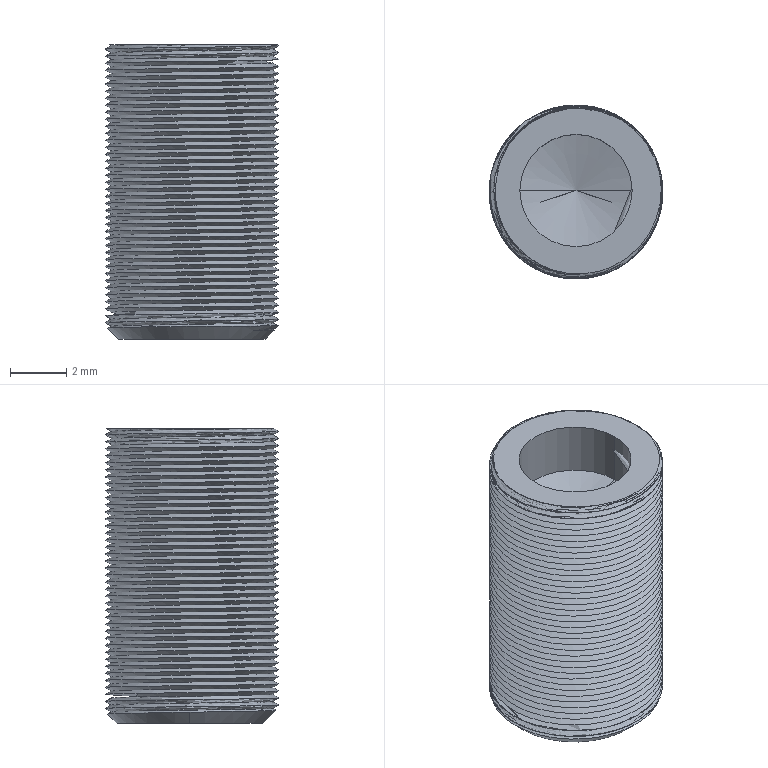Part | SolidWorks | features ICE 5, RevCut 4, Extrusion 1, Fillet 1, Helix 1, RefAxis 1, Sweep 1 | 1 solid | 18 faces | box 6.183 x 6.183 x 10.5 mm | volume 236.179 mm3 | plane 9 | cone 5 | cylinder 2 | spline 2 | commonest cylinder face diameters 4 x2